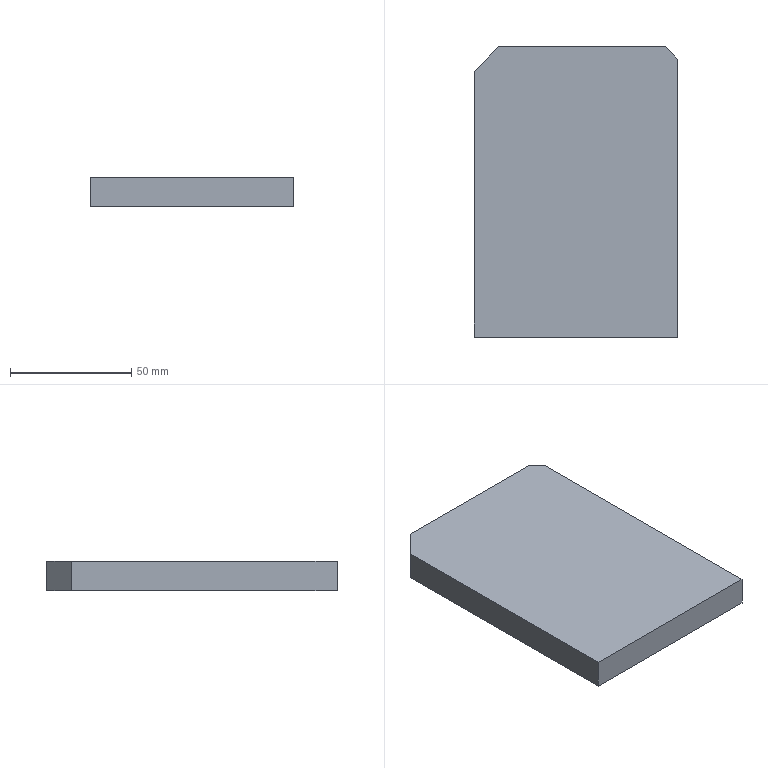Part | STEP file | ASND-0110-Body 1-1ww | 1 solid | 8 faces | box 84 x 119.7 x 12 mm | volume 119908 mm3 | plane 8
STEP:
#1=CARTESIAN_POINT('',(0.,0.,0.));
#2=DIRECTION('',(0.,0.,1.));
#3=DIRECTION('',(1.,0.,0.));
#4=AXIS2_PLACEMENT_3D('',#1,#2,#3);
#5=CARTESIAN_POINT('',(19.,119.7,0.));
#6=VERTEX_POINT('',#5);
#7=CARTESIAN_POINT('',(9.,109.7,0.));
#8=VERTEX_POINT('',#7);
#9=CARTESIAN_POINT('',(13.075,113.775,0.));
#10=DIRECTION('',(-0.7071,-0.7071,0.));
#11=VECTOR('',#10,1.);
#12=LINE('',#9,#11);
#13=CARTESIAN_POINT('',(14.,114.7,0.));
#14=DIRECTION('',(-0.7071,0.7071,0.));
#15=DIRECTION('',(0.5774,0.5774,0.5774));
#16=AXIS2_PLACEMENT_3D('',#13,#14,#15);
#17=PLANE('',#16);
#18=CARTESIAN_POINT('',(-1.068,-0.7553));
#19=DIRECTION('',(-0.8165,-0.5774));
#20=VECTOR('',#19,1.);
#21=LINE('',#18,#20);
#22=(GEOMETRIC_REPRESENTATION_CONTEXT(2)PARAMETRIC_REPRESENTATION_CONTEXT()REPRESENTATION_CONTEXT('',''));
#23=DEFINITIONAL_REPRESENTATION('',(#21),#22);
#24=PCURVE('',#17,#23);
#25=CARTESIAN_POINT('',(35.,60.,0.));
#26=DIRECTION('',(0.,0.,1.));
#27=DIRECTION('',(0.7071,0.7071,0.));
#28=AXIS2_PLACEMENT_3D('',#25,#26,#27);
#29=PLANE('',#28);
#30=CARTESIAN_POINT('',(22.521,53.528));
#31=DIRECTION('',(-1.,0.));
#32=VECTOR('',#31,1.);
#33=LINE('',#30,#32);
#34=(GEOMETRIC_REPRESENTATION_CONTEXT(2)PARAMETRIC_REPRESENTATION_CONTEXT()REPRESENTATION_CONTEXT('',''));
#35=DEFINITIONAL_REPRESENTATION('',(#33),#34);
#36=PCURVE('',#29,#35);
#37=SURFACE_CURVE('',#12,(#24,#36),.PCURVE_S1.);
#38=EDGE_CURVE('',#6,#8,#37,.T.);
#39=ORIENTED_EDGE('',*,*,#38,.T.);
#40=CARTESIAN_POINT('',(9.,109.7,12.));
#41=VERTEX_POINT('',#40);
#42=CARTESIAN_POINT('',(9.,109.7,0.));
#43=DIRECTION('',(0.,0.,1.));
#44=VECTOR('',#43,1.);
#45=LINE('',#42,#44);
#46=CARTESIAN_POINT('',(-5.774,-4.082));
#47=DIRECTION('',(0.5774,-0.8165));
#48=VECTOR('',#47,1.);
#49=LINE('',#46,#48);
#50=(GEOMETRIC_REPRESENTATION_CONTEXT(2)PARAMETRIC_REPRESENTATION_CONTEXT()REPRESENTATION_CONTEXT('',''));
#51=DEFINITIONAL_REPRESENTATION('',(#49),#50);
#52=PCURVE('',#17,#51);
#53=CARTESIAN_POINT('',(9.,0.,0.));
#54=DIRECTION('',(-1.,0.,0.));
#55=DIRECTION('',(0.,0.7071,0.7071));
#56=AXIS2_PLACEMENT_3D('',#53,#54,#55);
#57=PLANE('',#56);
#58=CARTESIAN_POINT('',(77.57,77.57));
#59=DIRECTION('',(0.7071,-0.7071));
#60=VECTOR('',#59,1.);
#61=LINE('',#58,#60);
#62=(GEOMETRIC_REPRESENTATION_CONTEXT(2)PARAMETRIC_REPRESENTATION_CONTEXT()REPRESENTATION_CONTEXT('',''));
#63=DEFINITIONAL_REPRESENTATION('',(#61),#62);
#64=PCURVE('',#57,#63);
#65=SURFACE_CURVE('',#45,(#52,#64),.PCURVE_S1.);
#66=EDGE_CURVE('',#8,#41,#65,.T.);
#67=ORIENTED_EDGE('',*,*,#66,.T.);
#68=CARTESIAN_POINT('',(19.,119.7,12.));
#69=VERTEX_POINT('',#68);
#70=CARTESIAN_POINT('',(13.075,113.775,12.));
#71=DIRECTION('',(0.7071,0.7071,0.));
#72=VECTOR('',#71,1.);
#73=LINE('',#70,#72);
#74=CARTESIAN_POINT('',(5.86,-10.553));
#75=DIRECTION('',(0.8165,0.5774));
#76=VECTOR('',#75,1.);
#77=LINE('',#74,#76);
#78=(GEOMETRIC_REPRESENTATION_CONTEXT(2)PARAMETRIC_REPRESENTATION_CONTEXT()REPRESENTATION_CONTEXT('',''));
#79=DEFINITIONAL_REPRESENTATION('',(#77),#78);
#80=PCURVE('',#17,#79);
#81=CARTESIAN_POINT('',(35.,60.,12.));
#82=DIRECTION('',(0.,0.,1.));
#83=DIRECTION('',(0.7071,0.7071,0.));
#84=AXIS2_PLACEMENT_3D('',#81,#82,#83);
#85=PLANE('',#84);
#86=CARTESIAN_POINT('',(22.521,53.528));
#87=DIRECTION('',(1.,0.));
#88=VECTOR('',#87,1.);
#89=LINE('',#86,#88);
#90=(GEOMETRIC_REPRESENTATION_CONTEXT(2)PARAMETRIC_REPRESENTATION_CONTEXT()REPRESENTATION_CONTEXT('',''));
#91=DEFINITIONAL_REPRESENTATION('',(#89),#90);
#92=PCURVE('',#85,#91);
#93=SURFACE_CURVE('',#73,(#80,#92),.PCURVE_S1.);
#94=EDGE_CURVE('',#41,#69,#93,.T.);
#95=ORIENTED_EDGE('',*,*,#94,.T.);
#96=CARTESIAN_POINT('',(19.,119.7,0.));
#97=DIRECTION('',(0.,0.,-1.));
#98=VECTOR('',#97,1.);
#99=LINE('',#96,#98);
#100=CARTESIAN_POINT('',(5.774,4.082));
#101=DIRECTION('',(-0.5774,0.8165));
#102=VECTOR('',#101,1.);
#103=LINE('',#100,#102);
#104=(GEOMETRIC_REPRESENTATION_CONTEXT(2)PARAMETRIC_REPRESENTATION_CONTEXT()REPRESENTATION_CONTEXT('',''));
#105=DEFINITIONAL_REPRESENTATION('',(#103),#104);
#106=PCURVE('',#17,#105);
#107=CARTESIAN_POINT('',(0.,119.7,0.));
#108=DIRECTION('',(0.,1.,0.));
#109=DIRECTION('',(0.7071,0.,0.7071));
#110=AXIS2_PLACEMENT_3D('',#107,#108,#109);
#111=PLANE('',#110);
#112=CARTESIAN_POINT('',(13.435,13.435));
#113=DIRECTION('',(-0.7071,0.7071));
#114=VECTOR('',#113,1.);
#115=LINE('',#112,#114);
#116=(GEOMETRIC_REPRESENTATION_CONTEXT(2)PARAMETRIC_REPRESENTATION_CONTEXT()REPRESENTATION_CONTEXT('',''));
#117=DEFINITIONAL_REPRESENTATION('',(#115),#116);
#118=PCURVE('',#111,#117);
#119=SURFACE_CURVE('',#99,(#106,#118),.PCURVE_S1.);
#120=EDGE_CURVE('',#69,#6,#119,.T.);
#121=ORIENTED_EDGE('',*,*,#120,.T.);
#122=EDGE_LOOP('',(#39,#67,#95,#121));
#123=FACE_BOUND('',#122,.T.);
#124=ADVANCED_FACE('',(#123),#17,.T.);
#125=ORIENTED_EDGE('',*,*,#94,.F.);
#126=CARTESIAN_POINT('',(9.,0.,12.));
#127=VERTEX_POINT('',#126);
#128=CARTESIAN_POINT('',(9.,5.,12.));
#129=DIRECTION('',(0.,1.,0.));
#130=VECTOR('',#129,1.);
#131=LINE('',#128,#130);
#132=CARTESIAN_POINT('',(-57.276,-20.506));
#133=DIRECTION('',(0.7071,0.7071));
#134=VECTOR('',#133,1.);
#135=LINE('',#132,#134);
#136=(GEOMETRIC_REPRESENTATION_CONTEXT(2)PARAMETRIC_REPRESENTATION_CONTEXT()REPRESENTATION_CONTEXT('',''));
#137=DEFINITIONAL_REPRESENTATION('',(#135),#136);
#138=PCURVE('',#85,#137);
#139=CARTESIAN_POINT('',(12.021,-4.95));
#140=DIRECTION('',(0.7071,0.7071));
#141=VECTOR('',#140,1.);
#142=LINE('',#139,#141);
#143=(GEOMETRIC_REPRESENTATION_CONTEXT(2)PARAMETRIC_REPRESENTATION_CONTEXT()REPRESENTATION_CONTEXT('',''));
#144=DEFINITIONAL_REPRESENTATION('',(#142),#143);
#145=PCURVE('',#57,#144);
#146=SURFACE_CURVE('',#131,(#138,#145),.PCURVE_S1.);
#147=EDGE_CURVE('',#127,#41,#146,.T.);
#148=ORIENTED_EDGE('',*,*,#147,.F.);
#149=CARTESIAN_POINT('',(93.,0.,12.));
#150=VERTEX_POINT('',#149);
#151=CARTESIAN_POINT('',(118.,0.,12.));
#152=DIRECTION('',(-1.,0.,0.));
#153=VECTOR('',#152,1.);
#154=LINE('',#151,#153);
#155=CARTESIAN_POINT('',(16.263,-101.116));
#156=DIRECTION('',(-0.7071,0.7071));
#157=VECTOR('',#156,1.);
#158=LINE('',#155,#157);
#159=(GEOMETRIC_REPRESENTATION_CONTEXT(2)PARAMETRIC_REPRESENTATION_CONTEXT()REPRESENTATION_CONTEXT('',''));
#160=DEFINITIONAL_REPRESENTATION('',(#158),#159);
#161=PCURVE('',#85,#160);
#162=CARTESIAN_POINT('',(70.,0.,0.));
#163=DIRECTION('',(0.,-1.,0.));
#164=DIRECTION('',(0.7071,0.,0.7071));
#165=AXIS2_PLACEMENT_3D('',#162,#163,#164);
#166=PLANE('',#165);
#167=CARTESIAN_POINT('',(42.426,-25.456));
#168=DIRECTION('',(-0.7071,0.7071));
#169=VECTOR('',#168,1.);
#170=LINE('',#167,#169);
#171=(GEOMETRIC_REPRESENTATION_CONTEXT(2)PARAMETRIC_REPRESENTATION_CONTEXT()REPRESENTATION_CONTEXT('',''));
#172=DEFINITIONAL_REPRESENTATION('',(#170),#171);
#173=PCURVE('',#166,#172);
#174=SURFACE_CURVE('',#154,(#161,#173),.PCURVE_S1.);
#175=EDGE_CURVE('',#150,#127,#174,.T.);
#176=ORIENTED_EDGE('',*,*,#175,.F.);
#177=CARTESIAN_POINT('',(93.,114.7,12.));
#178=VERTEX_POINT('',#177);
#179=CARTESIAN_POINT('',(93.,124.7,12.));
#180=DIRECTION('',(0.,-1.,0.));
#181=VECTOR('',#180,1.);
#182=LINE('',#179,#181);
#183=CARTESIAN_POINT('',(86.762,4.738));
#184=DIRECTION('',(-0.7071,-0.7071));
#185=VECTOR('',#184,1.);
#186=LINE('',#183,#185);
#187=(GEOMETRIC_REPRESENTATION_CONTEXT(2)PARAMETRIC_REPRESENTATION_CONTEXT()REPRESENTATION_CONTEXT('',''));
#188=DEFINITIONAL_REPRESENTATION('',(#186),#187);
#189=PCURVE('',#85,#188);
#190=CARTESIAN_POINT('',(93.,120.,0.));
#191=DIRECTION('',(1.,0.,0.));
#192=DIRECTION('',(0.,0.7071,0.7071));
#193=AXIS2_PLACEMENT_3D('',#190,#191,#192);
#194=PLANE('',#193);
#195=CARTESIAN_POINT('',(11.809,5.162));
#196=DIRECTION('',(-0.7071,0.7071));
#197=VECTOR('',#196,1.);
#198=LINE('',#195,#197);
#199=(GEOMETRIC_REPRESENTATION_CONTEXT(2)PARAMETRIC_REPRESENTATION_CONTEXT()REPRESENTATION_CONTEXT('',''));
#200=DEFINITIONAL_REPRESENTATION('',(#198),#199);
#201=PCURVE('',#194,#200);
#202=SURFACE_CURVE('',#182,(#189,#201),.PCURVE_S1.);
#203=EDGE_CURVE('',#178,#150,#202,.T.);
#204=ORIENTED_EDGE('',*,*,#203,.F.);
#205=CARTESIAN_POINT('',(88.,119.7,12.));
#206=VERTEX_POINT('',#205);
#207=CARTESIAN_POINT('',(88.,119.7,12.));
#208=DIRECTION('',(0.7071,-0.7071,0.));
#209=VECTOR('',#208,1.);
#210=LINE('',#207,#209);
#211=CARTESIAN_POINT('',(79.691,4.738));
#212=DIRECTION('',(0.,-1.));
#213=VECTOR('',#212,1.);
#214=LINE('',#211,#213);
#215=(GEOMETRIC_REPRESENTATION_CONTEXT(2)PARAMETRIC_REPRESENTATION_CONTEXT()REPRESENTATION_CONTEXT('',''));
#216=DEFINITIONAL_REPRESENTATION('',(#214),#215);
#217=PCURVE('',#85,#216);
#218=CARTESIAN_POINT('',(90.5,117.2,0.));
#219=DIRECTION('',(0.7071,0.7071,0.));
#220=DIRECTION('',(-0.5774,0.5774,0.5774));
#221=AXIS2_PLACEMENT_3D('',#218,#219,#220);
#222=PLANE('',#221);
#223=CARTESIAN_POINT('',(9.815,7.757));
#224=DIRECTION('',(-0.8165,0.5774));
#225=VECTOR('',#224,1.);
#226=LINE('',#223,#225);
#227=(GEOMETRIC_REPRESENTATION_CONTEXT(2)PARAMETRIC_REPRESENTATION_CONTEXT()REPRESENTATION_CONTEXT('',''));
#228=DEFINITIONAL_REPRESENTATION('',(#226),#227);
#229=PCURVE('',#222,#228);
#230=SURFACE_CURVE('',#210,(#217,#229),.PCURVE_S1.);
#231=EDGE_CURVE('',#206,#178,#230,.T.);
#232=ORIENTED_EDGE('',*,*,#231,.F.);
#233=CARTESIAN_POINT('',(5.,119.7,12.));
#234=DIRECTION('',(1.,0.,0.));
#235=VECTOR('',#234,1.);
#236=LINE('',#233,#235);
#237=CARTESIAN_POINT('',(21.001,63.427));
#238=DIRECTION('',(0.7071,-0.7071));
#239=VECTOR('',#238,1.);
#240=LINE('',#237,#239);
#241=(GEOMETRIC_REPRESENTATION_CONTEXT(2)PARAMETRIC_REPRESENTATION_CONTEXT()REPRESENTATION_CONTEXT('',''));
#242=DEFINITIONAL_REPRESENTATION('',(#240),#241);
#243=PCURVE('',#85,#242);
#244=CARTESIAN_POINT('',(12.021,-4.95));
#245=DIRECTION('',(0.7071,0.7071));
#246=VECTOR('',#245,1.);
#247=LINE('',#244,#246);
#248=(GEOMETRIC_REPRESENTATION_CONTEXT(2)PARAMETRIC_REPRESENTATION_CONTEXT()REPRESENTATION_CONTEXT('',''));
#249=DEFINITIONAL_REPRESENTATION('',(#247),#248);
#250=PCURVE('',#111,#249);
#251=SURFACE_CURVE('',#236,(#243,#250),.PCURVE_S1.);
#252=EDGE_CURVE('',#69,#206,#251,.T.);
#253=ORIENTED_EDGE('',*,*,#252,.F.);
#254=EDGE_LOOP('',(#125,#148,#176,#204,#232,#253));
#255=FACE_BOUND('',#254,.T.);
#256=ADVANCED_FACE('',(#255),#85,.T.);
#257=ORIENTED_EDGE('',*,*,#66,.F.);
#258=CARTESIAN_POINT('',(9.,0.,0.));
#259=VERTEX_POINT('',#258);
#260=CARTESIAN_POINT('',(9.,124.7,0.));
#261=DIRECTION('',(0.,-1.,0.));
#262=VECTOR('',#261,1.);
#263=LINE('',#260,#262);
#264=CARTESIAN_POINT('',(88.176,88.176));
#265=DIRECTION('',(-0.7071,-0.7071));
#266=VECTOR('',#265,1.);
#267=LINE('',#264,#266);
#268=(GEOMETRIC_REPRESENTATION_CONTEXT(2)PARAMETRIC_REPRESENTATION_CONTEXT()REPRESENTATION_CONTEXT('',''));
#269=DEFINITIONAL_REPRESENTATION('',(#267),#268);
#270=PCURVE('',#57,#269);
#271=CARTESIAN_POINT('',(27.365,64.135));
#272=DIRECTION('',(-0.7071,-0.7071));
#273=VECTOR('',#272,1.);
#274=LINE('',#271,#273);
#275=(GEOMETRIC_REPRESENTATION_CONTEXT(2)PARAMETRIC_REPRESENTATION_CONTEXT()REPRESENTATION_CONTEXT('',''));
#276=DEFINITIONAL_REPRESENTATION('',(#274),#275);
#277=PCURVE('',#29,#276);
#278=SURFACE_CURVE('',#263,(#270,#277),.PCURVE_S1.);
#279=EDGE_CURVE('',#8,#259,#278,.T.);
#280=ORIENTED_EDGE('',*,*,#279,.T.);
#281=CARTESIAN_POINT('',(9.,0.,0.));
#282=DIRECTION('',(0.,0.,1.));
#283=VECTOR('',#282,1.);
#284=LINE('',#281,#283);
#285=CARTESIAN_POINT('',(0.,0.));
#286=DIRECTION('',(0.7071,-0.7071));
#287=VECTOR('',#286,1.);
#288=LINE('',#285,#287);
#289=(GEOMETRIC_REPRESENTATION_CONTEXT(2)PARAMETRIC_REPRESENTATION_CONTEXT()REPRESENTATION_CONTEXT('',''));
#290=DEFINITIONAL_REPRESENTATION('',(#288),#289);
#291=PCURVE('',#57,#290);
#292=CARTESIAN_POINT('',(-43.134,43.134));
#293=DIRECTION('',(0.7071,0.7071));
#294=VECTOR('',#293,1.);
#295=LINE('',#292,#294);
#296=(GEOMETRIC_REPRESENTATION_CONTEXT(2)PARAMETRIC_REPRESENTATION_CONTEXT()REPRESENTATION_CONTEXT('',''));
#297=DEFINITIONAL_REPRESENTATION('',(#295),#296);
#298=PCURVE('',#166,#297);
#299=SURFACE_CURVE('',#284,(#291,#298),.PCURVE_S1.);
#300=EDGE_CURVE('',#259,#127,#299,.T.);
#301=ORIENTED_EDGE('',*,*,#300,.T.);
#302=ORIENTED_EDGE('',*,*,#147,.T.);
#303=EDGE_LOOP('',(#257,#280,#301,#302));
#304=FACE_BOUND('',#303,.T.);
#305=ADVANCED_FACE('',(#304),#57,.T.);
#306=ORIENTED_EDGE('',*,*,#300,.F.);
#307=CARTESIAN_POINT('',(93.,0.,0.));
#308=VERTEX_POINT('',#307);
#309=CARTESIAN_POINT('',(5.,0.,0.));
#310=DIRECTION('',(1.,0.,0.));
#311=VECTOR('',#310,1.);
#312=LINE('',#309,#311);
#313=CARTESIAN_POINT('',(-45.962,45.962));
#314=DIRECTION('',(0.7071,-0.7071));
#315=VECTOR('',#314,1.);
#316=LINE('',#313,#315);
#317=(GEOMETRIC_REPRESENTATION_CONTEXT(2)PARAMETRIC_REPRESENTATION_CONTEXT()REPRESENTATION_CONTEXT('',''));
#318=DEFINITIONAL_REPRESENTATION('',(#316),#317);
#319=PCURVE('',#166,#318);
#320=CARTESIAN_POINT('',(-63.64,-21.213));
#321=DIRECTION('',(0.7071,-0.7071));
#322=VECTOR('',#321,1.);
#323=LINE('',#320,#322);
#324=(GEOMETRIC_REPRESENTATION_CONTEXT(2)PARAMETRIC_REPRESENTATION_CONTEXT()REPRESENTATION_CONTEXT('',''));
#325=DEFINITIONAL_REPRESENTATION('',(#323),#324);
#326=PCURVE('',#29,#325);
#327=SURFACE_CURVE('',#312,(#319,#326),.PCURVE_S1.);
#328=EDGE_CURVE('',#259,#308,#327,.T.);
#329=ORIENTED_EDGE('',*,*,#328,.T.);
#330=CARTESIAN_POINT('',(93.,0.,10.));
#331=DIRECTION('',(0.,0.,-1.));
#332=VECTOR('',#331,1.);
#333=LINE('',#330,#332);
#334=CARTESIAN_POINT('',(23.335,-9.192));
#335=DIRECTION('',(-0.7071,-0.7071));
#336=VECTOR('',#335,1.);
#337=LINE('',#334,#336);
#338=(GEOMETRIC_REPRESENTATION_CONTEXT(2)PARAMETRIC_REPRESENTATION_CONTEXT()REPRESENTATION_CONTEXT('',''));
#339=DEFINITIONAL_REPRESENTATION('',(#337),#338);
#340=PCURVE('',#166,#339);
#341=CARTESIAN_POINT('',(-77.782,91.924));
#342=DIRECTION('',(-0.7071,-0.7071));
#343=VECTOR('',#342,1.);
#344=LINE('',#341,#343);
#345=(GEOMETRIC_REPRESENTATION_CONTEXT(2)PARAMETRIC_REPRESENTATION_CONTEXT()REPRESENTATION_CONTEXT('',''));
#346=DEFINITIONAL_REPRESENTATION('',(#344),#345);
#347=PCURVE('',#194,#346);
#348=SURFACE_CURVE('',#333,(#340,#347),.PCURVE_S1.);
#349=EDGE_CURVE('',#150,#308,#348,.T.);
#350=ORIENTED_EDGE('',*,*,#349,.F.);
#351=ORIENTED_EDGE('',*,*,#175,.T.);
#352=EDGE_LOOP('',(#306,#329,#350,#351));
#353=FACE_BOUND('',#352,.T.);
#354=ADVANCED_FACE('',(#353),#166,.T.);
#355=ORIENTED_EDGE('',*,*,#120,.F.);
#356=ORIENTED_EDGE('',*,*,#252,.T.);
#357=CARTESIAN_POINT('',(88.,119.7,0.));
#358=VERTEX_POINT('',#357);
#359=CARTESIAN_POINT('',(88.,119.7,0.));
#360=DIRECTION('',(0.,0.,1.));
#361=VECTOR('',#360,1.);
#362=LINE('',#359,#361);
#363=CARTESIAN_POINT('',(62.225,62.225));
#364=DIRECTION('',(0.7071,-0.7071));
#365=VECTOR('',#364,1.);
#366=LINE('',#363,#365);
#367=(GEOMETRIC_REPRESENTATION_CONTEXT(2)PARAMETRIC_REPRESENTATION_CONTEXT()REPRESENTATION_CONTEXT('',''));
#368=DEFINITIONAL_REPRESENTATION('',(#366),#367);
#369=PCURVE('',#111,#368);
#370=CARTESIAN_POINT('',(2.887,-2.041));
#371=DIRECTION('',(0.5774,0.8165));
#372=VECTOR('',#371,1.);
#373=LINE('',#370,#372);
#374=(GEOMETRIC_REPRESENTATION_CONTEXT(2)PARAMETRIC_REPRESENTATION_CONTEXT()REPRESENTATION_CONTEXT('',''));
#375=DEFINITIONAL_REPRESENTATION('',(#373),#374);
#376=PCURVE('',#222,#375);
#377=SURFACE_CURVE('',#362,(#369,#376),.PCURVE_S1.);
#378=EDGE_CURVE('',#358,#206,#377,.T.);
#379=ORIENTED_EDGE('',*,*,#378,.F.);
#380=CARTESIAN_POINT('',(113.,119.7,0.));
#381=DIRECTION('',(-1.,0.,0.));
#382=VECTOR('',#381,1.);
#383=LINE('',#380,#382);
#384=CARTESIAN_POINT('',(79.903,79.903));
#385=DIRECTION('',(-0.7071,-0.7071));
#386=VECTOR('',#385,1.);
#387=LINE('',#384,#386);
#388=(GEOMETRIC_REPRESENTATION_CONTEXT(2)PARAMETRIC_REPRESENTATION_CONTEXT()REPRESENTATION_CONTEXT('',''));
#389=DEFINITIONAL_REPRESENTATION('',(#387),#388);
#390=PCURVE('',#111,#389);
#391=CARTESIAN_POINT('',(97.369,-12.94));
#392=DIRECTION('',(-0.7071,0.7071));
#393=VECTOR('',#392,1.);
#394=LINE('',#391,#393);
#395=(GEOMETRIC_REPRESENTATION_CONTEXT(2)PARAMETRIC_REPRESENTATION_CONTEXT()REPRESENTATION_CONTEXT('',''));
#396=DEFINITIONAL_REPRESENTATION('',(#394),#395);
#397=PCURVE('',#29,#396);
#398=SURFACE_CURVE('',#383,(#390,#397),.PCURVE_S1.);
#399=EDGE_CURVE('',#358,#6,#398,.T.);
#400=ORIENTED_EDGE('',*,*,#399,.T.);
#401=EDGE_LOOP('',(#355,#356,#379,#400));
#402=FACE_BOUND('',#401,.T.);
#403=ADVANCED_FACE('',(#402),#111,.T.);
#404=ORIENTED_EDGE('',*,*,#38,.F.);
#405=ORIENTED_EDGE('',*,*,#399,.F.);
#406=CARTESIAN_POINT('',(93.,114.7,0.));
#407=VERTEX_POINT('',#406);
#408=CARTESIAN_POINT('',(93.,114.7,0.));
#409=DIRECTION('',(-0.7071,0.7071,0.));
#410=VECTOR('',#409,1.);
#411=LINE('',#408,#410);
#412=CARTESIAN_POINT('',(79.691,-2.333));
#413=DIRECTION('',(0.,1.));
#414=VECTOR('',#413,1.);
#415=LINE('',#412,#414);
#416=(GEOMETRIC_REPRESENTATION_CONTEXT(2)PARAMETRIC_REPRESENTATION_CONTEXT()REPRESENTATION_CONTEXT('',''));
#417=DEFINITIONAL_REPRESENTATION('',(#415),#416);
#418=PCURVE('',#29,#417);
#419=CARTESIAN_POINT('',(-2.887,2.041));
#420=DIRECTION('',(0.8165,-0.5774));
#421=VECTOR('',#420,1.);
#422=LINE('',#419,#421);
#423=(GEOMETRIC_REPRESENTATION_CONTEXT(2)PARAMETRIC_REPRESENTATION_CONTEXT()REPRESENTATION_CONTEXT('',''));
#424=DEFINITIONAL_REPRESENTATION('',(#422),#423);
#425=PCURVE('',#222,#424);
#426=SURFACE_CURVE('',#411,(#418,#425),.PCURVE_S1.);
#427=EDGE_CURVE('',#407,#358,#426,.T.);
#428=ORIENTED_EDGE('',*,*,#427,.F.);
#429=CARTESIAN_POINT('',(93.,0.,0.));
#430=DIRECTION('',(0.,1.,0.));
#431=VECTOR('',#430,1.);
#432=LINE('',#429,#431);
#433=CARTESIAN_POINT('',(-1.414,-83.439));
#434=DIRECTION('',(0.7071,0.7071));
#435=VECTOR('',#434,1.);
#436=LINE('',#433,#435);
#437=(GEOMETRIC_REPRESENTATION_CONTEXT(2)PARAMETRIC_REPRESENTATION_CONTEXT()REPRESENTATION_CONTEXT('',''));
#438=DEFINITIONAL_REPRESENTATION('',(#436),#437);
#439=PCURVE('',#29,#438);
#440=CARTESIAN_POINT('',(-84.853,84.853));
#441=DIRECTION('',(0.7071,-0.7071));
#442=VECTOR('',#441,1.);
#443=LINE('',#440,#442);
#444=(GEOMETRIC_REPRESENTATION_CONTEXT(2)PARAMETRIC_REPRESENTATION_CONTEXT()REPRESENTATION_CONTEXT('',''));
#445=DEFINITIONAL_REPRESENTATION('',(#443),#444);
#446=PCURVE('',#194,#445);
#447=SURFACE_CURVE('',#432,(#439,#446),.PCURVE_S1.);
#448=EDGE_CURVE('',#308,#407,#447,.T.);
#449=ORIENTED_EDGE('',*,*,#448,.F.);
#450=ORIENTED_EDGE('',*,*,#328,.F.);
#451=ORIENTED_EDGE('',*,*,#279,.F.);
#452=EDGE_LOOP('',(#404,#405,#428,#449,#450,#451));
#453=FACE_BOUND('',#452,.T.);
#454=ADVANCED_FACE('',(#453),#29,.F.);
#455=ORIENTED_EDGE('',*,*,#427,.T.);
#456=ORIENTED_EDGE('',*,*,#378,.T.);
#457=ORIENTED_EDGE('',*,*,#231,.T.);
#458=CARTESIAN_POINT('',(93.,114.7,10.));
#459=DIRECTION('',(0.,0.,-1.));
#460=VECTOR('',#459,1.);
#461=LINE('',#458,#460);
#462=CARTESIAN_POINT('',(2.887,10.206));
#463=DIRECTION('',(-0.5774,-0.8165));
#464=VECTOR('',#463,1.);
#465=LINE('',#462,#464);
#466=(GEOMETRIC_REPRESENTATION_CONTEXT(2)PARAMETRIC_REPRESENTATION_CONTEXT()REPRESENTATION_CONTEXT('',''));
#467=DEFINITIONAL_REPRESENTATION('',(#465),#466);
#468=PCURVE('',#222,#467);
#469=CARTESIAN_POINT('',(3.323,10.819));
#470=DIRECTION('',(-0.7071,-0.7071));
#471=VECTOR('',#470,1.);
#472=LINE('',#469,#471);
#473=(GEOMETRIC_REPRESENTATION_CONTEXT(2)PARAMETRIC_REPRESENTATION_CONTEXT()REPRESENTATION_CONTEXT('',''));
#474=DEFINITIONAL_REPRESENTATION('',(#472),#473);
#475=PCURVE('',#194,#474);
#476=SURFACE_CURVE('',#461,(#468,#475),.PCURVE_S1.);
#477=EDGE_CURVE('',#178,#407,#476,.T.);
#478=ORIENTED_EDGE('',*,*,#477,.T.);
#479=EDGE_LOOP('',(#455,#456,#457,#478));
#480=FACE_BOUND('',#479,.T.);
#481=ADVANCED_FACE('',(#480),#222,.T.);
#482=ORIENTED_EDGE('',*,*,#477,.F.);
#483=ORIENTED_EDGE('',*,*,#203,.T.);
#484=ORIENTED_EDGE('',*,*,#349,.T.);
#485=ORIENTED_EDGE('',*,*,#448,.T.);
#486=EDGE_LOOP('',(#482,#483,#484,#485));
#487=FACE_BOUND('',#486,.T.);
#488=ADVANCED_FACE('',(#487),#194,.T.);
#489=CLOSED_SHELL('',(#124,#256,#305,#354,#403,#454,#481,#488));
#490=MANIFOLD_SOLID_BREP('',#489);
#491=(LENGTH_UNIT()NAMED_UNIT(*)SI_UNIT(.MILLI.,.METRE.));
#492=UNCERTAINTY_MEASURE_WITH_UNIT(LENGTH_MEASURE(0.0000001),#491,'','');
#493=(NAMED_UNIT(*)PLANE_ANGLE_UNIT()SI_UNIT($,.RADIAN.));
#494=(NAMED_UNIT(*)SI_UNIT($,.STERADIAN.)SOLID_ANGLE_UNIT());
#495=(GEOMETRIC_REPRESENTATION_CONTEXT(3)GLOBAL_UNCERTAINTY_ASSIGNED_CONTEXT((#492))GLOBAL_UNIT_ASSIGNED_CONTEXT((#491,#493,#494))REPRESENTATION_CONTEXT('',''));
#496=ADVANCED_BREP_SHAPE_REPRESENTATION('',(#4,#490),#495);